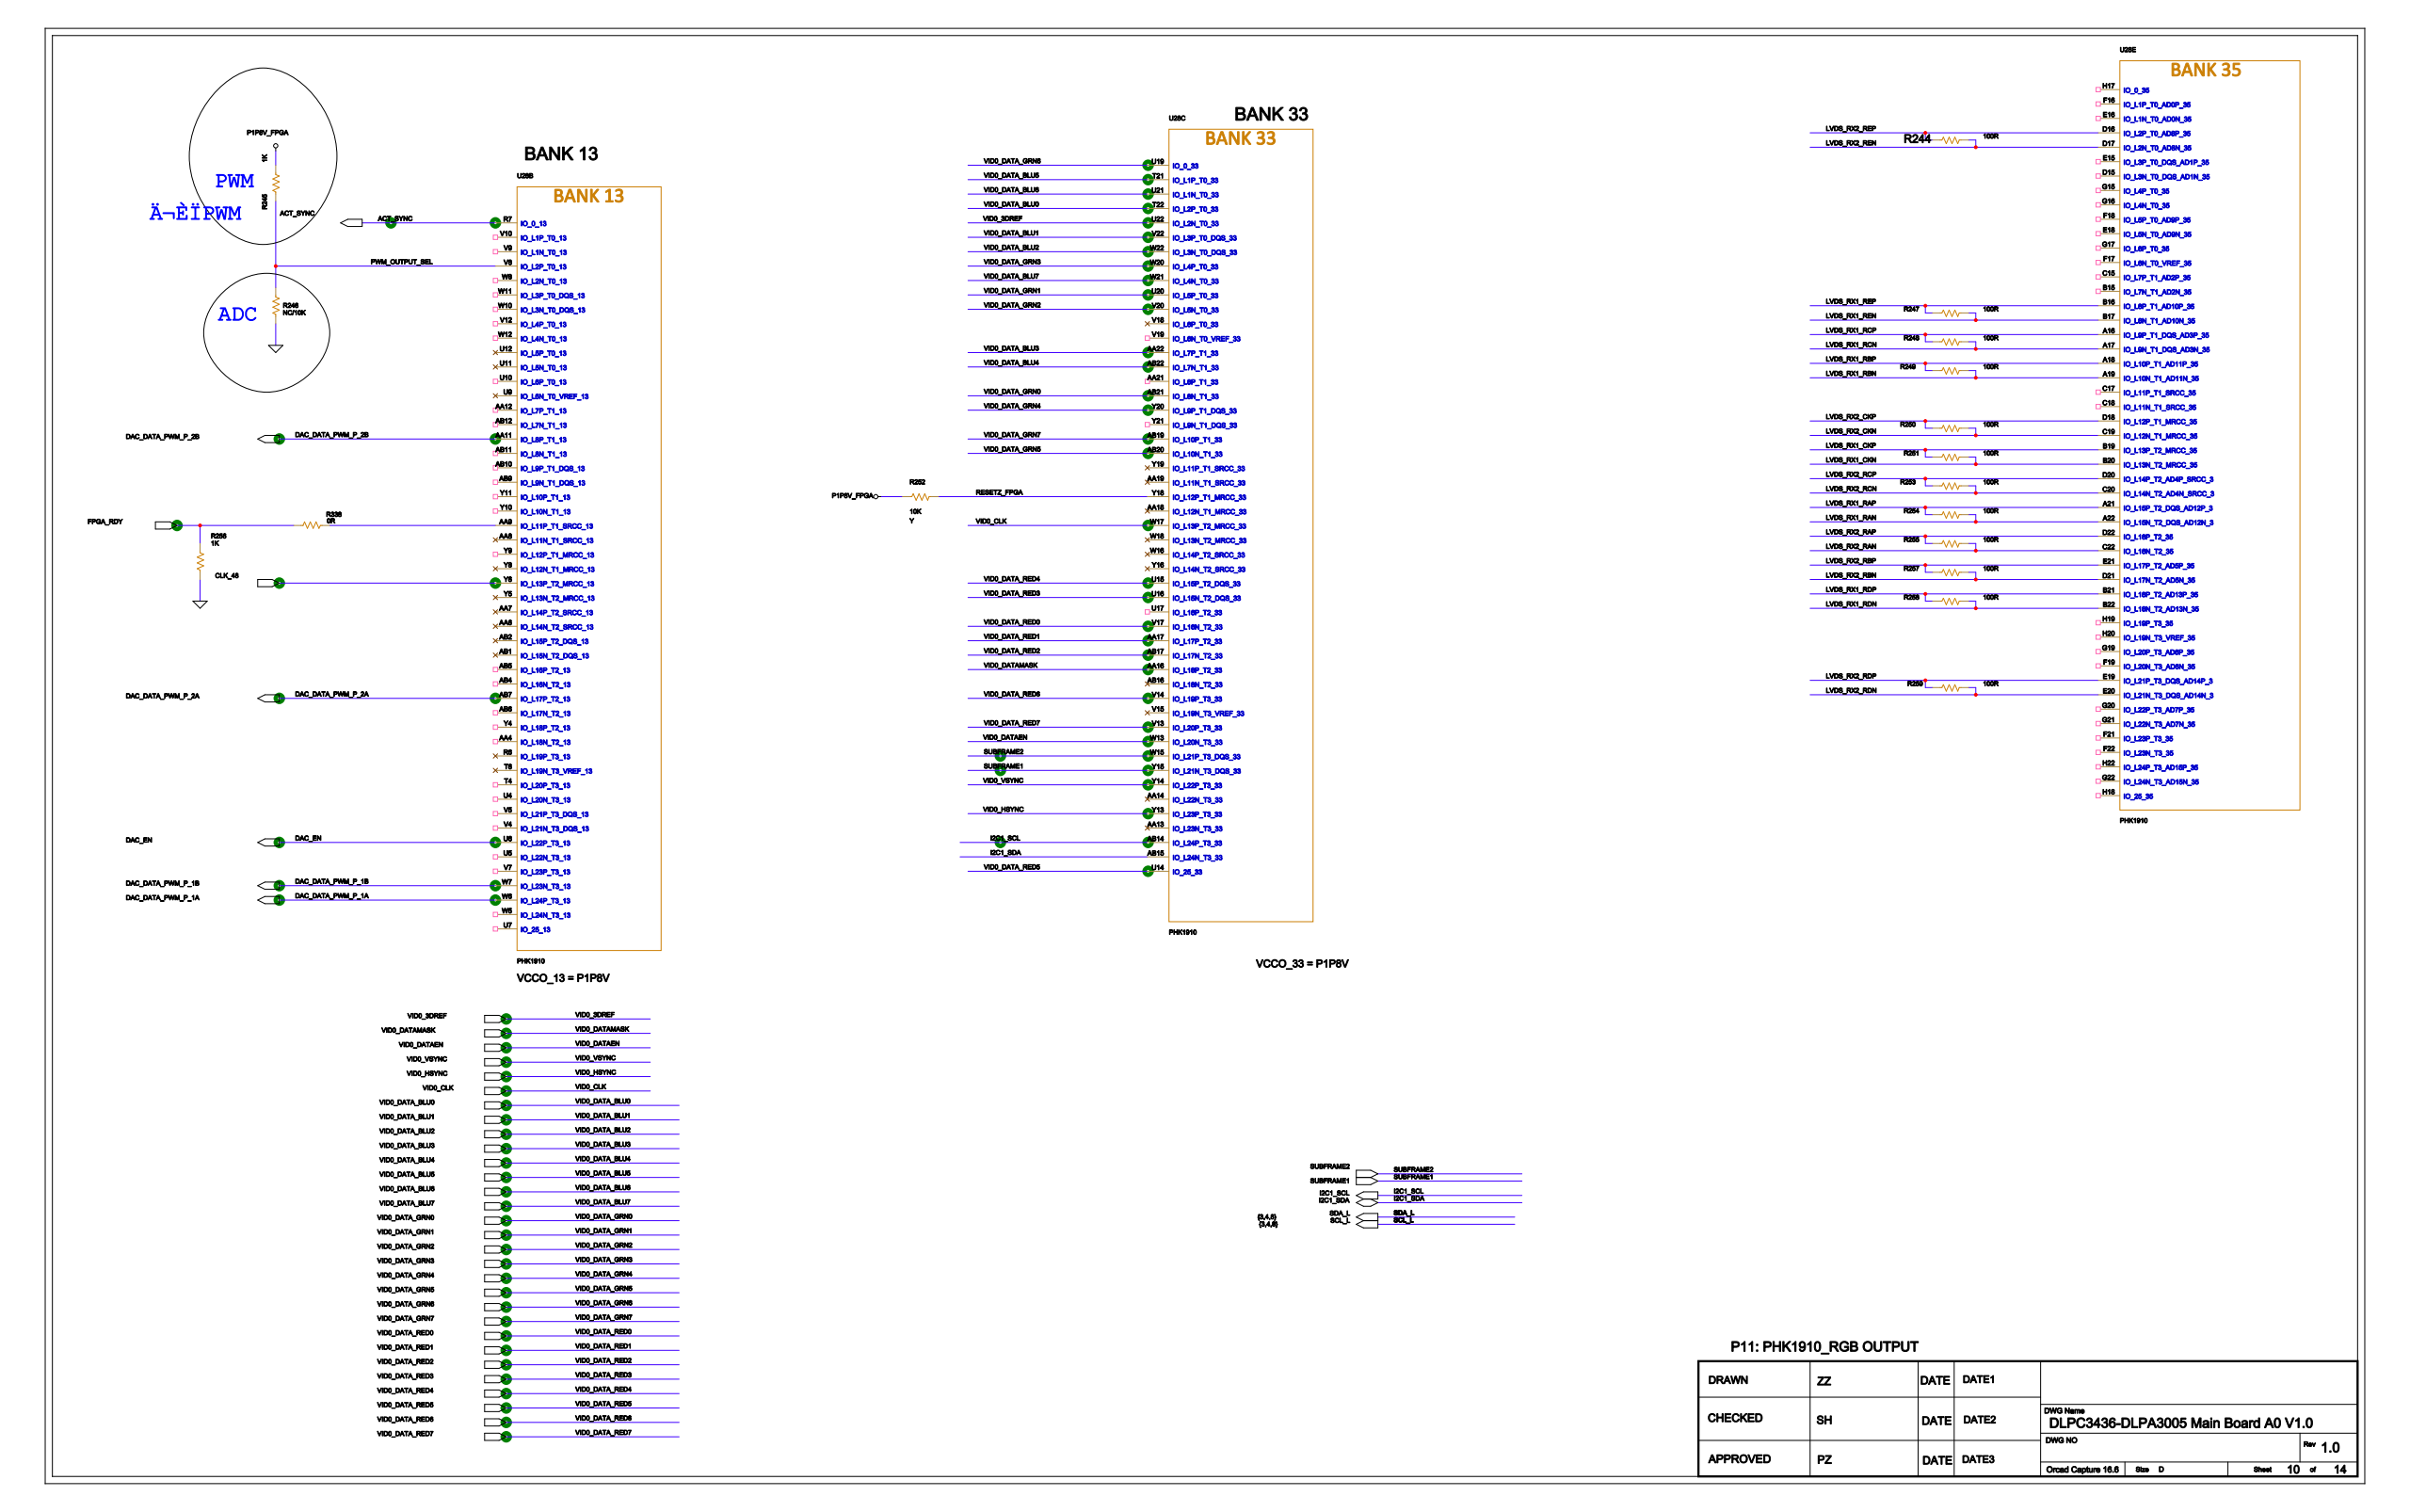Circuit board | Cadence Allegro | 1223 parts | 777 nets | one sheet of the schematic
Parts on this sheet (reference | value | footprint):
R244 | 100R | R0201
R245 | 1K | R0201
R246 | NC/10K | R0201
R247 | 100R | R0201
R248 | 100R | R0201
R249 | 100R | R0201
R250 | 100R | R0201
R251 | 100R | R0201
R252 | 10K | R0201
R253 | 100R | R0201
R254 | 100R | R0201
R255 | 100R | R0201
R256 | 1K | R0201
R257 | 100R | R0201
R258 | 100R | R0201
R259 | 100R | R0201
R338 | 0R | R0201
U12 | SC8886 | QFN32_5X5MM
U14 | SC2021 | QFN32_5X5MM
U16 | NTP8810 | QFN32_5X5MM
U28 | PHK1910 | XILINX_CLG484
Nets of these parts (net: part-pin ...):
GND: R246-2 R256-2 U12-14 U12-33 U14-10 U14-14 U14-33 U16-4 U16-13 U16-33
P1P8V_FPGA: R245-1 R252-2
CLK_48: U28-Y6
I2C1_SCL: U28-AB14
I2C1_SDA: U28-AB15
VID0_DATAMASK: U28-AA16
VID0_3DREF: U28-U22
RESETZ_FPGA: R252-1 U28-Y18
FPGA_RDY: R256-1 R338-1
N25602002: R338-2 U28-AA9
PWM_OUTPUT_SEL: R245-2 R246-1 U28-V8
DAC_EN: U28-U6
LVDS_RX2_REN: R244-1 U28-D17
LVDS_RX2_REP: R244-2 U28-D16
LVDS_RX1_REN: R247-1 U28-B17
LVDS_RX1_REP: R247-2 U28-B16
LVDS_RX1_RCN: R248-1 U28-A17
LVDS_RX1_RCP: R248-2 U28-A16
LVDS_RX1_RBN: R249-1 U28-A19
LVDS_RX1_RBP: R249-2 U28-A18
LVDS_RX2_CKN: R250-1 U28-C19
LVDS_RX2_CKP: R250-2 U28-D18
LVDS_RX1_CKN: R251-1 U28-B20
LVDS_RX1_CKP: R251-2 U28-B19
LVDS_RX2_RCN: R253-1 U28-C20
LVDS_RX2_RCP: R253-2 U28-D20
LVDS_RX1_RAN: R254-1 U28-A22
LVDS_RX1_RAP: R254-2 U28-A21
LVDS_RX2_RAN: R255-1 U28-C22
LVDS_RX2_RAP: R255-2 U28-D22
LVDS_RX2_RBN: R257-1 U28-D21
LVDS_RX2_RBP: R257-2 U28-E21
LVDS_RX1_RDN: R258-1 U28-B22
LVDS_RX1_RDP: R258-2 U28-B21
LVDS_RX2_RDN: R259-1 U28-E20
LVDS_RX2_RDP: R259-2 U28-E19
ACT_SYNC: U28-R7
DAC_DATA_PWM_P_2A: U28-AB7
DAC_DATA_PWM_P_1B: U28-W7
DAC_DATA_PWM_P_1A: U28-W6
DAC_DATA_PWM_P_2B: U28-AA11
VID0_DATA_GRN6: U28-U19
VID0_DATA_RED5: U28-U14
VID0_DATA_GRN5: U28-AB20
VID0_DATA_GRN7: U28-AB19
VID0_CLK: U28-W17
VID0_DATA_RED3: U28-U16
VID0_DATA_RED4: U28-U15
VID0_DATA_RED0: U28-V17
VID0_DATA_RED2: U28-AB17
VID0_DATA_RED1: U28-AA17
VID0_DATA_RED6: U28-V14
VID0_DATA_BLU6: U28-U21
VID0_DATA_BLU5: U28-T21
VID0_DATAEN: U28-W13
VID0_DATA_RED7: U28-V13
SUBFRAME1: U28-Y15
SUBFRAME2: U28-W15
VID0_VSYNC: U28-Y14
VID0_HSYNC: U28-Y13
VID0_DATA_BLU0: U28-T22
VID0_DATA_BLU2: U28-W22
VID0_DATA_BLU1: U28-V22
VID0_DATA_BLU7: U28-W21
VID0_DATA_GRN3: U28-W20
VID0_DATA_GRN2: U28-V20
VID0_DATA_GRN1: U28-U20
VID0_DATA_BLU4: U28-AB22
VID0_DATA_BLU3: U28-AA22
VID0_DATA_GRN0: U28-AB21
VID0_DATA_GRN4: U28-Y20